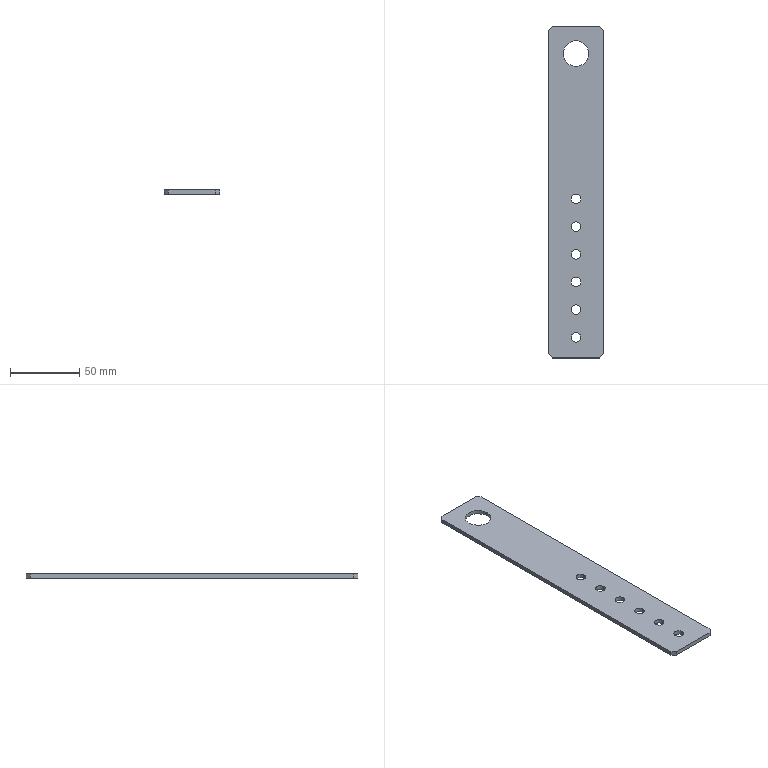Part | SolidWorks | features Extrusion 1 | 1 solid | 24 faces | box 40 x 240 x 3 mm | volume 27247 mm3 | cylinder 14 | plane 10 | commonest cylinder face diameters 7 x12 18.5 x2
STEP:
#1=CARTESIAN_POINT('',(-3.5,-5.,1.5));
#2=VERTEX_POINT('',#1);
#3=CARTESIAN_POINT('',(3.5,-5.,1.5));
#4=VERTEX_POINT('',#3);
#5=CARTESIAN_POINT('',(0.,-5.,1.5));
#6=DIRECTION('',(0.,0.,1.));
#7=DIRECTION('',(1.,0.,0.));
#8=AXIS2_PLACEMENT_3D('',#5,#6,#7);
#9=CIRCLE('',#8,3.5);
#10=EDGE_CURVE('',#2,#4,#9,.T.);
#11=ORIENTED_EDGE('',*,*,#10,.T.);
#12=CARTESIAN_POINT('',(3.5,-5.,-1.5));
#13=VERTEX_POINT('',#12);
#14=CARTESIAN_POINT('',(3.5,-5.,1.5));
#15=DIRECTION('',(0.,0.,-1.));
#16=VECTOR('',#15,1000.);
#17=LINE('',#14,#16);
#18=EDGE_CURVE('',#4,#13,#17,.T.);
#19=ORIENTED_EDGE('',*,*,#18,.T.);
#20=CARTESIAN_POINT('',(-3.5,-5.,-1.5));
#21=VERTEX_POINT('',#20);
#22=CARTESIAN_POINT('',(0.,-5.,-1.5));
#23=DIRECTION('',(0.,0.,1.));
#24=DIRECTION('',(1.,0.,0.));
#25=AXIS2_PLACEMENT_3D('',#22,#23,#24);
#26=CIRCLE('',#25,3.5);
#27=EDGE_CURVE('',#21,#13,#26,.T.);
#28=ORIENTED_EDGE('',*,*,#27,.F.);
#29=CARTESIAN_POINT('',(-3.5,-5.,1.5));
#30=DIRECTION('',(0.,0.,-1.));
#31=VECTOR('',#30,1000.);
#32=LINE('',#29,#31);
#33=EDGE_CURVE('',#2,#21,#32,.T.);
#34=ORIENTED_EDGE('',*,*,#33,.F.);
#35=EDGE_LOOP('',(#11,#19,#28,#34));
#36=FACE_OUTER_BOUND('',#35,.T.);
#37=CARTESIAN_POINT('',(0.,-5.,1.5));
#38=DIRECTION('',(0.,0.,-1.));
#39=DIRECTION('',(-1.,0.,0.));
#40=AXIS2_PLACEMENT_3D('',#37,#38,#39);
#41=CYLINDRICAL_SURFACE('',#40,3.5);
#42=ADVANCED_FACE('',(#36),#41,.F.);
#43=CARTESIAN_POINT('',(-3.5,-25.,1.5));
#44=VERTEX_POINT('',#43);
#45=CARTESIAN_POINT('',(3.5,-25.,1.5));
#46=VERTEX_POINT('',#45);
#47=CARTESIAN_POINT('',(0.,-25.,1.5));
#48=DIRECTION('',(0.,0.,1.));
#49=DIRECTION('',(1.,0.,0.));
#50=AXIS2_PLACEMENT_3D('',#47,#48,#49);
#51=CIRCLE('',#50,3.5);
#52=EDGE_CURVE('',#44,#46,#51,.T.);
#53=ORIENTED_EDGE('',*,*,#52,.T.);
#54=CARTESIAN_POINT('',(3.5,-25.,-1.5));
#55=VERTEX_POINT('',#54);
#56=CARTESIAN_POINT('',(3.5,-25.,1.5));
#57=DIRECTION('',(0.,0.,-1.));
#58=VECTOR('',#57,1000.);
#59=LINE('',#56,#58);
#60=EDGE_CURVE('',#46,#55,#59,.T.);
#61=ORIENTED_EDGE('',*,*,#60,.T.);
#62=CARTESIAN_POINT('',(-3.5,-25.,-1.5));
#63=VERTEX_POINT('',#62);
#64=CARTESIAN_POINT('',(0.,-25.,-1.5));
#65=DIRECTION('',(0.,0.,1.));
#66=DIRECTION('',(1.,0.,0.));
#67=AXIS2_PLACEMENT_3D('',#64,#65,#66);
#68=CIRCLE('',#67,3.5);
#69=EDGE_CURVE('',#63,#55,#68,.T.);
#70=ORIENTED_EDGE('',*,*,#69,.F.);
#71=CARTESIAN_POINT('',(-3.5,-25.,1.5));
#72=DIRECTION('',(0.,0.,-1.));
#73=VECTOR('',#72,1000.);
#74=LINE('',#71,#73);
#75=EDGE_CURVE('',#44,#63,#74,.T.);
#76=ORIENTED_EDGE('',*,*,#75,.F.);
#77=EDGE_LOOP('',(#53,#61,#70,#76));
#78=FACE_OUTER_BOUND('',#77,.T.);
#79=CARTESIAN_POINT('',(0.,-25.,1.5));
#80=DIRECTION('',(0.,0.,-1.));
#81=DIRECTION('',(-1.,0.,0.));
#82=AXIS2_PLACEMENT_3D('',#79,#80,#81);
#83=CYLINDRICAL_SURFACE('',#82,3.5);
#84=ADVANCED_FACE('',(#78),#83,.F.);
#85=CARTESIAN_POINT('',(-3.5,-45.,1.5));
#86=VERTEX_POINT('',#85);
#87=CARTESIAN_POINT('',(3.5,-45.,1.5));
#88=VERTEX_POINT('',#87);
#89=CARTESIAN_POINT('',(0.,-45.,1.5));
#90=DIRECTION('',(0.,0.,1.));
#91=DIRECTION('',(1.,0.,0.));
#92=AXIS2_PLACEMENT_3D('',#89,#90,#91);
#93=CIRCLE('',#92,3.5);
#94=EDGE_CURVE('',#86,#88,#93,.T.);
#95=ORIENTED_EDGE('',*,*,#94,.T.);
#96=CARTESIAN_POINT('',(3.5,-45.,-1.5));
#97=VERTEX_POINT('',#96);
#98=CARTESIAN_POINT('',(3.5,-45.,1.5));
#99=DIRECTION('',(0.,0.,-1.));
#100=VECTOR('',#99,1000.);
#101=LINE('',#98,#100);
#102=EDGE_CURVE('',#88,#97,#101,.T.);
#103=ORIENTED_EDGE('',*,*,#102,.T.);
#104=CARTESIAN_POINT('',(-3.5,-45.,-1.5));
#105=VERTEX_POINT('',#104);
#106=CARTESIAN_POINT('',(0.,-45.,-1.5));
#107=DIRECTION('',(0.,0.,1.));
#108=DIRECTION('',(1.,0.,0.));
#109=AXIS2_PLACEMENT_3D('',#106,#107,#108);
#110=CIRCLE('',#109,3.5);
#111=EDGE_CURVE('',#105,#97,#110,.T.);
#112=ORIENTED_EDGE('',*,*,#111,.F.);
#113=CARTESIAN_POINT('',(-3.5,-45.,1.5));
#114=DIRECTION('',(0.,0.,-1.));
#115=VECTOR('',#114,1000.);
#116=LINE('',#113,#115);
#117=EDGE_CURVE('',#86,#105,#116,.T.);
#118=ORIENTED_EDGE('',*,*,#117,.F.);
#119=EDGE_LOOP('',(#95,#103,#112,#118));
#120=FACE_OUTER_BOUND('',#119,.T.);
#121=CARTESIAN_POINT('',(0.,-45.,1.5));
#122=DIRECTION('',(0.,0.,-1.));
#123=DIRECTION('',(-1.,0.,0.));
#124=AXIS2_PLACEMENT_3D('',#121,#122,#123);
#125=CYLINDRICAL_SURFACE('',#124,3.5);
#126=ADVANCED_FACE('',(#120),#125,.F.);
#127=CARTESIAN_POINT('',(-3.5,-65.,1.5));
#128=VERTEX_POINT('',#127);
#129=CARTESIAN_POINT('',(3.5,-65.,1.5));
#130=VERTEX_POINT('',#129);
#131=CARTESIAN_POINT('',(0.,-65.,1.5));
#132=DIRECTION('',(0.,0.,1.));
#133=DIRECTION('',(1.,0.,0.));
#134=AXIS2_PLACEMENT_3D('',#131,#132,#133);
#135=CIRCLE('',#134,3.5);
#136=EDGE_CURVE('',#128,#130,#135,.T.);
#137=ORIENTED_EDGE('',*,*,#136,.T.);
#138=CARTESIAN_POINT('',(3.5,-65.,-1.5));
#139=VERTEX_POINT('',#138);
#140=CARTESIAN_POINT('',(3.5,-65.,1.5));
#141=DIRECTION('',(0.,0.,-1.));
#142=VECTOR('',#141,1000.);
#143=LINE('',#140,#142);
#144=EDGE_CURVE('',#130,#139,#143,.T.);
#145=ORIENTED_EDGE('',*,*,#144,.T.);
#146=CARTESIAN_POINT('',(-3.5,-65.,-1.5));
#147=VERTEX_POINT('',#146);
#148=CARTESIAN_POINT('',(0.,-65.,-1.5));
#149=DIRECTION('',(0.,0.,1.));
#150=DIRECTION('',(1.,0.,0.));
#151=AXIS2_PLACEMENT_3D('',#148,#149,#150);
#152=CIRCLE('',#151,3.5);
#153=EDGE_CURVE('',#147,#139,#152,.T.);
#154=ORIENTED_EDGE('',*,*,#153,.F.);
#155=CARTESIAN_POINT('',(-3.5,-65.,1.5));
#156=DIRECTION('',(0.,0.,-1.));
#157=VECTOR('',#156,1000.);
#158=LINE('',#155,#157);
#159=EDGE_CURVE('',#128,#147,#158,.T.);
#160=ORIENTED_EDGE('',*,*,#159,.F.);
#161=EDGE_LOOP('',(#137,#145,#154,#160));
#162=FACE_OUTER_BOUND('',#161,.T.);
#163=CARTESIAN_POINT('',(0.,-65.,1.5));
#164=DIRECTION('',(0.,0.,-1.));
#165=DIRECTION('',(-1.,0.,0.));
#166=AXIS2_PLACEMENT_3D('',#163,#164,#165);
#167=CYLINDRICAL_SURFACE('',#166,3.5);
#168=ADVANCED_FACE('',(#162),#167,.F.);
#169=CARTESIAN_POINT('',(-3.5,-85.,1.5));
#170=VERTEX_POINT('',#169);
#171=CARTESIAN_POINT('',(3.5,-85.,1.5));
#172=VERTEX_POINT('',#171);
#173=CARTESIAN_POINT('',(0.,-85.,1.5));
#174=DIRECTION('',(0.,0.,1.));
#175=DIRECTION('',(1.,0.,0.));
#176=AXIS2_PLACEMENT_3D('',#173,#174,#175);
#177=CIRCLE('',#176,3.5);
#178=EDGE_CURVE('',#170,#172,#177,.T.);
#179=ORIENTED_EDGE('',*,*,#178,.T.);
#180=CARTESIAN_POINT('',(3.5,-85.,-1.5));
#181=VERTEX_POINT('',#180);
#182=CARTESIAN_POINT('',(3.5,-85.,1.5));
#183=DIRECTION('',(0.,0.,-1.));
#184=VECTOR('',#183,1000.);
#185=LINE('',#182,#184);
#186=EDGE_CURVE('',#172,#181,#185,.T.);
#187=ORIENTED_EDGE('',*,*,#186,.T.);
#188=CARTESIAN_POINT('',(-3.5,-85.,-1.5));
#189=VERTEX_POINT('',#188);
#190=CARTESIAN_POINT('',(0.,-85.,-1.5));
#191=DIRECTION('',(0.,0.,1.));
#192=DIRECTION('',(1.,0.,0.));
#193=AXIS2_PLACEMENT_3D('',#190,#191,#192);
#194=CIRCLE('',#193,3.5);
#195=EDGE_CURVE('',#189,#181,#194,.T.);
#196=ORIENTED_EDGE('',*,*,#195,.F.);
#197=CARTESIAN_POINT('',(-3.5,-85.,1.5));
#198=DIRECTION('',(0.,0.,-1.));
#199=VECTOR('',#198,1000.);
#200=LINE('',#197,#199);
#201=EDGE_CURVE('',#170,#189,#200,.T.);
#202=ORIENTED_EDGE('',*,*,#201,.F.);
#203=EDGE_LOOP('',(#179,#187,#196,#202));
#204=FACE_OUTER_BOUND('',#203,.T.);
#205=CARTESIAN_POINT('',(0.,-85.,1.5));
#206=DIRECTION('',(0.,0.,-1.));
#207=DIRECTION('',(-1.,0.,0.));
#208=AXIS2_PLACEMENT_3D('',#205,#206,#207);
#209=CYLINDRICAL_SURFACE('',#208,3.5);
#210=ADVANCED_FACE('',(#204),#209,.F.);
#211=CARTESIAN_POINT('',(-3.5,-105.,1.5));
#212=VERTEX_POINT('',#211);
#213=CARTESIAN_POINT('',(3.5,-105.,1.5));
#214=VERTEX_POINT('',#213);
#215=CARTESIAN_POINT('',(0.,-105.,1.5));
#216=DIRECTION('',(0.,0.,1.));
#217=DIRECTION('',(1.,0.,0.));
#218=AXIS2_PLACEMENT_3D('',#215,#216,#217);
#219=CIRCLE('',#218,3.5);
#220=EDGE_CURVE('',#212,#214,#219,.T.);
#221=ORIENTED_EDGE('',*,*,#220,.T.);
#222=CARTESIAN_POINT('',(3.5,-105.,-1.5));
#223=VERTEX_POINT('',#222);
#224=CARTESIAN_POINT('',(3.5,-105.,1.5));
#225=DIRECTION('',(0.,0.,-1.));
#226=VECTOR('',#225,1000.);
#227=LINE('',#224,#226);
#228=EDGE_CURVE('',#214,#223,#227,.T.);
#229=ORIENTED_EDGE('',*,*,#228,.T.);
#230=CARTESIAN_POINT('',(-3.5,-105.,-1.5));
#231=VERTEX_POINT('',#230);
#232=CARTESIAN_POINT('',(0.,-105.,-1.5));
#233=DIRECTION('',(0.,0.,1.));
#234=DIRECTION('',(1.,0.,0.));
#235=AXIS2_PLACEMENT_3D('',#232,#233,#234);
#236=CIRCLE('',#235,3.5);
#237=EDGE_CURVE('',#231,#223,#236,.T.);
#238=ORIENTED_EDGE('',*,*,#237,.F.);
#239=CARTESIAN_POINT('',(-3.5,-105.,1.5));
#240=DIRECTION('',(0.,0.,-1.));
#241=VECTOR('',#240,1000.);
#242=LINE('',#239,#241);
#243=EDGE_CURVE('',#212,#231,#242,.T.);
#244=ORIENTED_EDGE('',*,*,#243,.F.);
#245=EDGE_LOOP('',(#221,#229,#238,#244));
#246=FACE_OUTER_BOUND('',#245,.T.);
#247=CARTESIAN_POINT('',(0.,-105.,1.5));
#248=DIRECTION('',(0.,0.,-1.));
#249=DIRECTION('',(-1.,0.,0.));
#250=AXIS2_PLACEMENT_3D('',#247,#248,#249);
#251=CYLINDRICAL_SURFACE('',#250,3.5);
#252=ADVANCED_FACE('',(#246),#251,.F.);
#253=CARTESIAN_POINT('',(-9.25,100.,1.5));
#254=VERTEX_POINT('',#253);
#255=CARTESIAN_POINT('',(9.25,100.,1.5));
#256=VERTEX_POINT('',#255);
#257=CARTESIAN_POINT('',(0.,100.,1.5));
#258=DIRECTION('',(0.,0.,1.));
#259=DIRECTION('',(1.,0.,0.));
#260=AXIS2_PLACEMENT_3D('',#257,#258,#259);
#261=CIRCLE('',#260,9.25);
#262=EDGE_CURVE('',#254,#256,#261,.T.);
#263=ORIENTED_EDGE('',*,*,#262,.T.);
#264=CARTESIAN_POINT('',(9.25,100.,-1.5));
#265=VERTEX_POINT('',#264);
#266=CARTESIAN_POINT('',(9.25,100.,1.5));
#267=DIRECTION('',(0.,0.,-1.));
#268=VECTOR('',#267,1000.);
#269=LINE('',#266,#268);
#270=EDGE_CURVE('',#256,#265,#269,.T.);
#271=ORIENTED_EDGE('',*,*,#270,.T.);
#272=CARTESIAN_POINT('',(-9.25,100.,-1.5));
#273=VERTEX_POINT('',#272);
#274=CARTESIAN_POINT('',(0.,100.,-1.5));
#275=DIRECTION('',(0.,0.,1.));
#276=DIRECTION('',(1.,0.,0.));
#277=AXIS2_PLACEMENT_3D('',#274,#275,#276);
#278=CIRCLE('',#277,9.25);
#279=EDGE_CURVE('',#273,#265,#278,.T.);
#280=ORIENTED_EDGE('',*,*,#279,.F.);
#281=CARTESIAN_POINT('',(-9.25,100.,1.5));
#282=DIRECTION('',(0.,0.,-1.));
#283=VECTOR('',#282,1000.);
#284=LINE('',#281,#283);
#285=EDGE_CURVE('',#254,#273,#284,.T.);
#286=ORIENTED_EDGE('',*,*,#285,.F.);
#287=EDGE_LOOP('',(#263,#271,#280,#286));
#288=FACE_OUTER_BOUND('',#287,.T.);
#289=CARTESIAN_POINT('',(0.,100.,1.5));
#290=DIRECTION('',(0.,0.,-1.));
#291=DIRECTION('',(-1.,0.,0.));
#292=AXIS2_PLACEMENT_3D('',#289,#290,#291);
#293=CYLINDRICAL_SURFACE('',#292,9.25);
#294=ADVANCED_FACE('',(#288),#293,.F.);
#295=ORIENTED_EDGE('',*,*,#52,.F.);
#296=CARTESIAN_POINT('',(0.,-25.,1.5));
#297=DIRECTION('',(0.,0.,1.));
#298=DIRECTION('',(1.,0.,0.));
#299=AXIS2_PLACEMENT_3D('',#296,#297,#298);
#300=CIRCLE('',#299,3.5);
#301=EDGE_CURVE('',#46,#44,#300,.T.);
#302=ORIENTED_EDGE('',*,*,#301,.F.);
#303=EDGE_LOOP('',(#295,#302));
#304=FACE_BOUND('',#303,.T.);
#305=ORIENTED_EDGE('',*,*,#136,.F.);
#306=CARTESIAN_POINT('',(0.,-65.,1.5));
#307=DIRECTION('',(0.,0.,1.));
#308=DIRECTION('',(1.,0.,0.));
#309=AXIS2_PLACEMENT_3D('',#306,#307,#308);
#310=CIRCLE('',#309,3.5);
#311=EDGE_CURVE('',#130,#128,#310,.T.);
#312=ORIENTED_EDGE('',*,*,#311,.F.);
#313=EDGE_LOOP('',(#305,#312));
#314=FACE_BOUND('',#313,.T.);
#315=ORIENTED_EDGE('',*,*,#220,.F.);
#316=CARTESIAN_POINT('',(0.,-105.,1.5));
#317=DIRECTION('',(0.,0.,1.));
#318=DIRECTION('',(1.,0.,0.));
#319=AXIS2_PLACEMENT_3D('',#316,#317,#318);
#320=CIRCLE('',#319,3.5);
#321=EDGE_CURVE('',#214,#212,#320,.T.);
#322=ORIENTED_EDGE('',*,*,#321,.F.);
#323=EDGE_LOOP('',(#315,#322));
#324=FACE_BOUND('',#323,.T.);
#325=CARTESIAN_POINT('',(-20.,117.,1.5));
#326=VERTEX_POINT('',#325);
#327=CARTESIAN_POINT('',(-20.,-117.,1.5));
#328=VERTEX_POINT('',#327);
#329=CARTESIAN_POINT('',(-20.,-117.,1.5));
#330=DIRECTION('',(0.,-1.,0.));
#331=VECTOR('',#330,1000.);
#332=LINE('',#329,#331);
#333=EDGE_CURVE('',#326,#328,#332,.T.);
#334=ORIENTED_EDGE('',*,*,#333,.T.);
#335=CARTESIAN_POINT('',(-17.,-120.,1.5));
#336=VERTEX_POINT('',#335);
#337=CARTESIAN_POINT('',(-17.,-120.,1.5));
#338=DIRECTION('',(0.7071,-0.7071,0.));
#339=VECTOR('',#338,1000.);
#340=LINE('',#337,#339);
#341=EDGE_CURVE('',#328,#336,#340,.T.);
#342=ORIENTED_EDGE('',*,*,#341,.T.);
#343=CARTESIAN_POINT('',(17.,-120.,1.5));
#344=VERTEX_POINT('',#343);
#345=CARTESIAN_POINT('',(17.,-120.,1.5));
#346=DIRECTION('',(1.,0.,0.));
#347=VECTOR('',#346,1000.);
#348=LINE('',#345,#347);
#349=EDGE_CURVE('',#336,#344,#348,.T.);
#350=ORIENTED_EDGE('',*,*,#349,.T.);
#351=CARTESIAN_POINT('',(20.,-117.,1.5));
#352=VERTEX_POINT('',#351);
#353=CARTESIAN_POINT('',(17.,-120.,1.5));
#354=DIRECTION('',(0.7071,0.7071,0.));
#355=VECTOR('',#354,1000.);
#356=LINE('',#353,#355);
#357=EDGE_CURVE('',#344,#352,#356,.T.);
#358=ORIENTED_EDGE('',*,*,#357,.T.);
#359=CARTESIAN_POINT('',(20.,117.,1.5));
#360=VERTEX_POINT('',#359);
#361=CARTESIAN_POINT('',(20.,-117.,1.5));
#362=DIRECTION('',(0.,1.,0.));
#363=VECTOR('',#362,1000.);
#364=LINE('',#361,#363);
#365=EDGE_CURVE('',#352,#360,#364,.T.);
#366=ORIENTED_EDGE('',*,*,#365,.T.);
#367=CARTESIAN_POINT('',(17.,120.,1.5));
#368=VERTEX_POINT('',#367);
#369=CARTESIAN_POINT('',(20.,117.,1.5));
#370=DIRECTION('',(-0.7071,0.7071,0.));
#371=VECTOR('',#370,1000.);
#372=LINE('',#369,#371);
#373=EDGE_CURVE('',#360,#368,#372,.T.);
#374=ORIENTED_EDGE('',*,*,#373,.T.);
#375=CARTESIAN_POINT('',(-17.,120.,1.5));
#376=VERTEX_POINT('',#375);
#377=CARTESIAN_POINT('',(17.,120.,1.5));
#378=DIRECTION('',(-1.,0.,0.));
#379=VECTOR('',#378,1000.);
#380=LINE('',#377,#379);
#381=EDGE_CURVE('',#368,#376,#380,.T.);
#382=ORIENTED_EDGE('',*,*,#381,.T.);
#383=CARTESIAN_POINT('',(-20.,117.,1.5));
#384=DIRECTION('',(-0.7071,-0.7071,0.));
#385=VECTOR('',#384,1000.);
#386=LINE('',#383,#385);
#387=EDGE_CURVE('',#376,#326,#386,.T.);
#388=ORIENTED_EDGE('',*,*,#387,.T.);
#389=EDGE_LOOP('',(#334,#342,#350,#358,#366,#374,#382,#388));
#390=FACE_OUTER_BOUND('',#389,.T.);
#391=ORIENTED_EDGE('',*,*,#262,.F.);
#392=CARTESIAN_POINT('',(0.,100.,1.5));
#393=DIRECTION('',(0.,0.,1.));
#394=DIRECTION('',(1.,0.,0.));
#395=AXIS2_PLACEMENT_3D('',#392,#393,#394);
#396=CIRCLE('',#395,9.25);
#397=EDGE_CURVE('',#256,#254,#396,.T.);
#398=ORIENTED_EDGE('',*,*,#397,.F.);
#399=EDGE_LOOP('',(#391,#398));
#400=FACE_BOUND('',#399,.T.);
#401=ORIENTED_EDGE('',*,*,#178,.F.);
#402=CARTESIAN_POINT('',(0.,-85.,1.5));
#403=DIRECTION('',(0.,0.,1.));
#404=DIRECTION('',(1.,0.,0.));
#405=AXIS2_PLACEMENT_3D('',#402,#403,#404);
#406=CIRCLE('',#405,3.5);
#407=EDGE_CURVE('',#172,#170,#406,.T.);
#408=ORIENTED_EDGE('',*,*,#407,.F.);
#409=EDGE_LOOP('',(#401,#408));
#410=FACE_BOUND('',#409,.T.);
#411=ORIENTED_EDGE('',*,*,#94,.F.);
#412=CARTESIAN_POINT('',(0.,-45.,1.5));
#413=DIRECTION('',(0.,0.,1.));
#414=DIRECTION('',(1.,0.,0.));
#415=AXIS2_PLACEMENT_3D('',#412,#413,#414);
#416=CIRCLE('',#415,3.5);
#417=EDGE_CURVE('',#88,#86,#416,.T.);
#418=ORIENTED_EDGE('',*,*,#417,.F.);
#419=EDGE_LOOP('',(#411,#418));
#420=FACE_BOUND('',#419,.T.);
#421=ORIENTED_EDGE('',*,*,#10,.F.);
#422=CARTESIAN_POINT('',(0.,-5.,1.5));
#423=DIRECTION('',(0.,0.,1.));
#424=DIRECTION('',(1.,0.,0.));
#425=AXIS2_PLACEMENT_3D('',#422,#423,#424);
#426=CIRCLE('',#425,3.5);
#427=EDGE_CURVE('',#4,#2,#426,.T.);
#428=ORIENTED_EDGE('',*,*,#427,.F.);
#429=EDGE_LOOP('',(#421,#428));
#430=FACE_BOUND('',#429,.T.);
#431=CARTESIAN_POINT('',(0.,0.,1.5));
#432=DIRECTION('',(0.,0.,1.));
#433=DIRECTION('',(1.,0.,0.));
#434=AXIS2_PLACEMENT_3D('',#431,#432,#433);
#435=PLANE('',#434);
#436=ADVANCED_FACE('',(#304,#314,#324,#390,#400,#410,#420,#430),#435,.T.);
#437=CARTESIAN_POINT('',(-20.,117.,-1.5));
#438=VERTEX_POINT('',#437);
#439=CARTESIAN_POINT('',(-20.,-117.,-1.5));
#440=VERTEX_POINT('',#439);
#441=CARTESIAN_POINT('',(-20.,-117.,-1.5));
#442=DIRECTION('',(0.,-1.,0.));
#443=VECTOR('',#442,1000.);
#444=LINE('',#441,#443);
#445=EDGE_CURVE('',#438,#440,#444,.T.);
#446=ORIENTED_EDGE('',*,*,#445,.F.);
#447=CARTESIAN_POINT('',(-17.,120.,-1.5));
#448=VERTEX_POINT('',#447);
#449=CARTESIAN_POINT('',(-20.,117.,-1.5));
#450=DIRECTION('',(-0.7071,-0.7071,0.));
#451=VECTOR('',#450,1000.);
#452=LINE('',#449,#451);
#453=EDGE_CURVE('',#448,#438,#452,.T.);
#454=ORIENTED_EDGE('',*,*,#453,.F.);
#455=CARTESIAN_POINT('',(17.,120.,-1.5));
#456=VERTEX_POINT('',#455);
#457=CARTESIAN_POINT('',(17.,120.,-1.5));
#458=DIRECTION('',(-1.,0.,0.));
#459=VECTOR('',#458,1000.);
#460=LINE('',#457,#459);
#461=EDGE_CURVE('',#456,#448,#460,.T.);
#462=ORIENTED_EDGE('',*,*,#461,.F.);
#463=CARTESIAN_POINT('',(20.,117.,-1.5));
#464=VERTEX_POINT('',#463);
#465=CARTESIAN_POINT('',(20.,117.,-1.5));
#466=DIRECTION('',(-0.7071,0.7071,0.));
#467=VECTOR('',#466,1000.);
#468=LINE('',#465,#467);
#469=EDGE_CURVE('',#464,#456,#468,.T.);
#470=ORIENTED_EDGE('',*,*,#469,.F.);
#471=CARTESIAN_POINT('',(20.,-117.,-1.5));
#472=VERTEX_POINT('',#471);
#473=CARTESIAN_POINT('',(20.,-117.,-1.5));
#474=DIRECTION('',(0.,1.,0.));
#475=VECTOR('',#474,1000.);
#476=LINE('',#473,#475);
#477=EDGE_CURVE('',#472,#464,#476,.T.);
#478=ORIENTED_EDGE('',*,*,#477,.F.);
#479=CARTESIAN_POINT('',(17.,-120.,-1.5));
#480=VERTEX_POINT('',#479);
#481=CARTESIAN_POINT('',(17.,-120.,-1.5));
#482=DIRECTION('',(0.7071,0.7071,0.));
#483=VECTOR('',#482,1000.);
#484=LINE('',#481,#483);
#485=EDGE_CURVE('',#480,#472,#484,.T.);
#486=ORIENTED_EDGE('',*,*,#485,.F.);
#487=CARTESIAN_POINT('',(-17.,-120.,-1.5));
#488=VERTEX_POINT('',#487);
#489=CARTESIAN_POINT('',(17.,-120.,-1.5));
#490=DIRECTION('',(1.,0.,0.));
#491=VECTOR('',#490,1000.);
#492=LINE('',#489,#491);
#493=EDGE_CURVE('',#488,#480,#492,.T.);
#494=ORIENTED_EDGE('',*,*,#493,.F.);
#495=CARTESIAN_POINT('',(-17.,-120.,-1.5));
#496=DIRECTION('',(0.7071,-0.7071,0.));
#497=VECTOR('',#496,1000.);
#498=LINE('',#495,#497);
#499=EDGE_CURVE('',#440,#488,#498,.T.);
#500=ORIENTED_EDGE('',*,*,#499,.F.);
#501=EDGE_LOOP('',(#446,#454,#462,#470,#478,#486,#494,#500));
#502=FACE_OUTER_BOUND('',#501,.T.);
#503=ORIENTED_EDGE('',*,*,#279,.T.);
#504=CARTESIAN_POINT('',(0.,100.,-1.5));
#505=DIRECTION('',(0.,0.,1.));
#506=DIRECTION('',(1.,0.,0.));
#507=AXIS2_PLACEMENT_3D('',#504,#505,#506);
#508=CIRCLE('',#507,9.25);
#509=EDGE_CURVE('',#265,#273,#508,.T.);
#510=ORIENTED_EDGE('',*,*,#509,.T.);
#511=EDGE_LOOP('',(#503,#510));
#512=FACE_BOUND('',#511,.T.);
#513=ORIENTED_EDGE('',*,*,#237,.T.);
#514=CARTESIAN_POINT('',(0.,-105.,-1.5));
#515=DIRECTION('',(0.,0.,1.));
#516=DIRECTION('',(1.,0.,0.));
#517=AXIS2_PLACEMENT_3D('',#514,#515,#516);
#518=CIRCLE('',#517,3.5);
#519=EDGE_CURVE('',#223,#231,#518,.T.);
#520=ORIENTED_EDGE('',*,*,#519,.T.);
#521=EDGE_LOOP('',(#513,#520));
#522=FACE_BOUND('',#521,.T.);
#523=ORIENTED_EDGE('',*,*,#195,.T.);
#524=CARTESIAN_POINT('',(0.,-85.,-1.5));
#525=DIRECTION('',(0.,0.,1.));
#526=DIRECTION('',(1.,0.,0.));
#527=AXIS2_PLACEMENT_3D('',#524,#525,#526);
#528=CIRCLE('',#527,3.5);
#529=EDGE_CURVE('',#181,#189,#528,.T.);
#530=ORIENTED_EDGE('',*,*,#529,.T.);
#531=EDGE_LOOP('',(#523,#530));
#532=FACE_BOUND('',#531,.T.);
#533=ORIENTED_EDGE('',*,*,#153,.T.);
#534=CARTESIAN_POINT('',(0.,-65.,-1.5));
#535=DIRECTION('',(0.,0.,1.));
#536=DIRECTION('',(1.,0.,0.));
#537=AXIS2_PLACEMENT_3D('',#534,#535,#536);
#538=CIRCLE('',#537,3.5);
#539=EDGE_CURVE('',#139,#147,#538,.T.);
#540=ORIENTED_EDGE('',*,*,#539,.T.);
#541=EDGE_LOOP('',(#533,#540));
#542=FACE_BOUND('',#541,.T.);
#543=ORIENTED_EDGE('',*,*,#111,.T.);
#544=CARTESIAN_POINT('',(0.,-45.,-1.5));
#545=DIRECTION('',(0.,0.,1.));
#546=DIRECTION('',(1.,0.,0.));
#547=AXIS2_PLACEMENT_3D('',#544,#545,#546);
#548=CIRCLE('',#547,3.5);
#549=EDGE_CURVE('',#97,#105,#548,.T.);
#550=ORIENTED_EDGE('',*,*,#549,.T.);
#551=EDGE_LOOP('',(#543,#550));
#552=FACE_BOUND('',#551,.T.);
#553=ORIENTED_EDGE('',*,*,#69,.T.);
#554=CARTESIAN_POINT('',(0.,-25.,-1.5));
#555=DIRECTION('',(0.,0.,1.));
#556=DIRECTION('',(1.,0.,0.));
#557=AXIS2_PLACEMENT_3D('',#554,#555,#556);
#558=CIRCLE('',#557,3.5);
#559=EDGE_CURVE('',#55,#63,#558,.T.);
#560=ORIENTED_EDGE('',*,*,#559,.T.);
#561=EDGE_LOOP('',(#553,#560));
#562=FACE_BOUND('',#561,.T.);
#563=ORIENTED_EDGE('',*,*,#27,.T.);
#564=CARTESIAN_POINT('',(0.,-5.,-1.5));
#565=DIRECTION('',(0.,0.,1.));
#566=DIRECTION('',(1.,0.,0.));
#567=AXIS2_PLACEMENT_3D('',#564,#565,#566);
#568=CIRCLE('',#567,3.5);
#569=EDGE_CURVE('',#13,#21,#568,.T.);
#570=ORIENTED_EDGE('',*,*,#569,.T.);
#571=EDGE_LOOP('',(#563,#570));
#572=FACE_BOUND('',#571,.T.);
#573=CARTESIAN_POINT('',(0.,0.,-1.5));
#574=DIRECTION('',(0.,0.,1.));
#575=DIRECTION('',(1.,0.,0.));
#576=AXIS2_PLACEMENT_3D('',#573,#574,#575);
#577=PLANE('',#576);
#578=ADVANCED_FACE('',(#502,#512,#522,#532,#542,#552,#562,#572),#577,.F.);
#579=ORIENTED_EDGE('',*,*,#445,.T.);
#580=CARTESIAN_POINT('',(-20.,-117.,1.5));
#581=DIRECTION('',(0.,0.,-1.));
#582=VECTOR('',#581,1000.);
#583=LINE('',#580,#582);
#584=EDGE_CURVE('',#328,#440,#583,.T.);
#585=ORIENTED_EDGE('',*,*,#584,.F.);
#586=ORIENTED_EDGE('',*,*,#333,.F.);
#587=CARTESIAN_POINT('',(-20.,117.,1.5));
#588=DIRECTION('',(0.,0.,-1.));
#589=VECTOR('',#588,1000.);
#590=LINE('',#587,#589);
#591=EDGE_CURVE('',#326,#438,#590,.T.);
#592=ORIENTED_EDGE('',*,*,#591,.T.);
#593=EDGE_LOOP('',(#579,#585,#586,#592));
#594=FACE_OUTER_BOUND('',#593,.T.);
#595=CARTESIAN_POINT('',(-20.,-117.,1.5));
#596=DIRECTION('',(1.,0.,0.));
#597=DIRECTION('',(0.,0.,-1.));
#598=AXIS2_PLACEMENT_3D('',#595,#596,#597);
#599=PLANE('',#598);
#600=ADVANCED_FACE('',(#594),#599,.F.);
#601=ORIENTED_EDGE('',*,*,#499,.T.);
#602=CARTESIAN_POINT('',(-17.,-120.,1.5));
#603=DIRECTION('',(0.,0.,-1.));
#604=VECTOR('',#603,1000.);
#605=LINE('',#602,#604);
#606=EDGE_CURVE('',#336,#488,#605,.T.);
#607=ORIENTED_EDGE('',*,*,#606,.F.);
#608=ORIENTED_EDGE('',*,*,#341,.F.);
#609=ORIENTED_EDGE('',*,*,#584,.T.);
#610=EDGE_LOOP('',(#601,#607,#608,#609));
#611=FACE_OUTER_BOUND('',#610,.T.);
#612=CARTESIAN_POINT('',(-17.,-120.,1.5));
#613=DIRECTION('',(0.7071,0.7071,0.));
#614=DIRECTION('',(-0.7071,0.7071,0.));
#615=AXIS2_PLACEMENT_3D('',#612,#613,#614);
#616=PLANE('',#615);
#617=ADVANCED_FACE('',(#611),#616,.F.);
#618=ORIENTED_EDGE('',*,*,#493,.T.);
#619=CARTESIAN_POINT('',(17.,-120.,1.5));
#620=DIRECTION('',(0.,0.,-1.));
#621=VECTOR('',#620,1000.);
#622=LINE('',#619,#621);
#623=EDGE_CURVE('',#344,#480,#622,.T.);
#624=ORIENTED_EDGE('',*,*,#623,.F.);
#625=ORIENTED_EDGE('',*,*,#349,.F.);
#626=ORIENTED_EDGE('',*,*,#606,.T.);
#627=EDGE_LOOP('',(#618,#624,#625,#626));
#628=FACE_OUTER_BOUND('',#627,.T.);
#629=CARTESIAN_POINT('',(17.,-120.,1.5));
#630=DIRECTION('',(0.,1.,0.));
#631=DIRECTION('',(0.,0.,1.));
#632=AXIS2_PLACEMENT_3D('',#629,#630,#631);
#633=PLANE('',#632);
#634=ADVANCED_FACE('',(#628),#633,.F.);
#635=ORIENTED_EDGE('',*,*,#485,.T.);
#636=CARTESIAN_POINT('',(20.,-117.,1.5));
#637=DIRECTION('',(0.,0.,-1.));
#638=VECTOR('',#637,1000.);
#639=LINE('',#636,#638);
#640=EDGE_CURVE('',#352,#472,#639,.T.);
#641=ORIENTED_EDGE('',*,*,#640,.F.);
#642=ORIENTED_EDGE('',*,*,#357,.F.);
#643=ORIENTED_EDGE('',*,*,#623,.T.);
#644=EDGE_LOOP('',(#635,#641,#642,#643));
#645=FACE_OUTER_BOUND('',#644,.T.);
#646=CARTESIAN_POINT('',(17.,-120.,1.5));
#647=DIRECTION('',(-0.7071,0.7071,0.));
#648=DIRECTION('',(-0.7071,-0.7071,0.));
#649=AXIS2_PLACEMENT_3D('',#646,#647,#648);
#650=PLANE('',#649);
#651=ADVANCED_FACE('',(#645),#650,.F.);
#652=ORIENTED_EDGE('',*,*,#477,.T.);
#653=CARTESIAN_POINT('',(20.,117.,1.5));
#654=DIRECTION('',(0.,0.,-1.));
#655=VECTOR('',#654,1000.);
#656=LINE('',#653,#655);
#657=EDGE_CURVE('',#360,#464,#656,.T.);
#658=ORIENTED_EDGE('',*,*,#657,.F.);
#659=ORIENTED_EDGE('',*,*,#365,.F.);
#660=ORIENTED_EDGE('',*,*,#640,.T.);
#661=EDGE_LOOP('',(#652,#658,#659,#660));
#662=FACE_OUTER_BOUND('',#661,.T.);
#663=CARTESIAN_POINT('',(20.,-117.,1.5));
#664=DIRECTION('',(-1.,0.,0.));
#665=DIRECTION('',(0.,0.,1.));
#666=AXIS2_PLACEMENT_3D('',#663,#664,#665);
#667=PLANE('',#666);
#668=ADVANCED_FACE('',(#662),#667,.F.);
#669=ORIENTED_EDGE('',*,*,#469,.T.);
#670=CARTESIAN_POINT('',(17.,120.,1.5));
#671=DIRECTION('',(0.,0.,-1.));
#672=VECTOR('',#671,1000.);
#673=LINE('',#670,#672);
#674=EDGE_CURVE('',#368,#456,#673,.T.);
#675=ORIENTED_EDGE('',*,*,#674,.F.);
#676=ORIENTED_EDGE('',*,*,#373,.F.);
#677=ORIENTED_EDGE('',*,*,#657,.T.);
#678=EDGE_LOOP('',(#669,#675,#676,#677));
#679=FACE_OUTER_BOUND('',#678,.T.);
#680=CARTESIAN_POINT('',(20.,117.,1.5));
#681=DIRECTION('',(-0.7071,-0.7071,0.));
#682=DIRECTION('',(0.7071,-0.7071,0.));
#683=AXIS2_PLACEMENT_3D('',#680,#681,#682);
#684=PLANE('',#683);
#685=ADVANCED_FACE('',(#679),#684,.F.);
#686=ORIENTED_EDGE('',*,*,#461,.T.);
#687=CARTESIAN_POINT('',(-17.,120.,1.5));
#688=DIRECTION('',(0.,0.,-1.));
#689=VECTOR('',#688,1000.);
#690=LINE('',#687,#689);
#691=EDGE_CURVE('',#376,#448,#690,.T.);
#692=ORIENTED_EDGE('',*,*,#691,.F.);
#693=ORIENTED_EDGE('',*,*,#381,.F.);
#694=ORIENTED_EDGE('',*,*,#674,.T.);
#695=EDGE_LOOP('',(#686,#692,#693,#694));
#696=FACE_OUTER_BOUND('',#695,.T.);
#697=CARTESIAN_POINT('',(17.,120.,1.5));
#698=DIRECTION('',(0.,-1.,0.));
#699=DIRECTION('',(1.,0.,0.));
#700=AXIS2_PLACEMENT_3D('',#697,#698,#699);
#701=PLANE('',#700);
#702=ADVANCED_FACE('',(#696),#701,.F.);
#703=ORIENTED_EDGE('',*,*,#453,.T.);
#704=ORIENTED_EDGE('',*,*,#591,.F.);
#705=ORIENTED_EDGE('',*,*,#387,.F.);
#706=ORIENTED_EDGE('',*,*,#691,.T.);
#707=EDGE_LOOP('',(#703,#704,#705,#706));
#708=FACE_OUTER_BOUND('',#707,.T.);
#709=CARTESIAN_POINT('',(-20.,117.,1.5));
#710=DIRECTION('',(0.7071,-0.7071,0.));
#711=DIRECTION('',(0.7071,0.7071,0.));
#712=AXIS2_PLACEMENT_3D('',#709,#710,#711);
#713=PLANE('',#712);
#714=ADVANCED_FACE('',(#708),#713,.F.);
#715=ORIENTED_EDGE('',*,*,#270,.F.);
#716=ORIENTED_EDGE('',*,*,#397,.T.);
#717=ORIENTED_EDGE('',*,*,#285,.T.);
#718=ORIENTED_EDGE('',*,*,#509,.F.);
#719=EDGE_LOOP('',(#715,#716,#717,#718));
#720=FACE_OUTER_BOUND('',#719,.T.);
#721=CARTESIAN_POINT('',(0.,100.,1.5));
#722=DIRECTION('',(0.,0.,-1.));
#723=DIRECTION('',(-1.,0.,0.));
#724=AXIS2_PLACEMENT_3D('',#721,#722,#723);
#725=CYLINDRICAL_SURFACE('',#724,9.25);
#726=ADVANCED_FACE('',(#720),#725,.F.);
#727=ORIENTED_EDGE('',*,*,#228,.F.);
#728=ORIENTED_EDGE('',*,*,#321,.T.);
#729=ORIENTED_EDGE('',*,*,#243,.T.);
#730=ORIENTED_EDGE('',*,*,#519,.F.);
#731=EDGE_LOOP('',(#727,#728,#729,#730));
#732=FACE_OUTER_BOUND('',#731,.T.);
#733=CARTESIAN_POINT('',(0.,-105.,1.5));
#734=DIRECTION('',(0.,0.,-1.));
#735=DIRECTION('',(-1.,0.,0.));
#736=AXIS2_PLACEMENT_3D('',#733,#734,#735);
#737=CYLINDRICAL_SURFACE('',#736,3.5);
#738=ADVANCED_FACE('',(#732),#737,.F.);
#739=ORIENTED_EDGE('',*,*,#186,.F.);
#740=ORIENTED_EDGE('',*,*,#407,.T.);
#741=ORIENTED_EDGE('',*,*,#201,.T.);
#742=ORIENTED_EDGE('',*,*,#529,.F.);
#743=EDGE_LOOP('',(#739,#740,#741,#742));
#744=FACE_OUTER_BOUND('',#743,.T.);
#745=CARTESIAN_POINT('',(0.,-85.,1.5));
#746=DIRECTION('',(0.,0.,-1.));
#747=DIRECTION('',(-1.,0.,0.));
#748=AXIS2_PLACEMENT_3D('',#745,#746,#747);
#749=CYLINDRICAL_SURFACE('',#748,3.5);
#750=ADVANCED_FACE('',(#744),#749,.F.);
#751=ORIENTED_EDGE('',*,*,#144,.F.);
#752=ORIENTED_EDGE('',*,*,#311,.T.);
#753=ORIENTED_EDGE('',*,*,#159,.T.);
#754=ORIENTED_EDGE('',*,*,#539,.F.);
#755=EDGE_LOOP('',(#751,#752,#753,#754));
#756=FACE_OUTER_BOUND('',#755,.T.);
#757=CARTESIAN_POINT('',(0.,-65.,1.5));
#758=DIRECTION('',(0.,0.,-1.));
#759=DIRECTION('',(-1.,0.,0.));
#760=AXIS2_PLACEMENT_3D('',#757,#758,#759);
#761=CYLINDRICAL_SURFACE('',#760,3.5);
#762=ADVANCED_FACE('',(#756),#761,.F.);
#763=ORIENTED_EDGE('',*,*,#102,.F.);
#764=ORIENTED_EDGE('',*,*,#417,.T.);
#765=ORIENTED_EDGE('',*,*,#117,.T.);
#766=ORIENTED_EDGE('',*,*,#549,.F.);
#767=EDGE_LOOP('',(#763,#764,#765,#766));
#768=FACE_OUTER_BOUND('',#767,.T.);
#769=CARTESIAN_POINT('',(0.,-45.,1.5));
#770=DIRECTION('',(0.,0.,-1.));
#771=DIRECTION('',(-1.,0.,0.));
#772=AXIS2_PLACEMENT_3D('',#769,#770,#771);
#773=CYLINDRICAL_SURFACE('',#772,3.5);
#774=ADVANCED_FACE('',(#768),#773,.F.);
#775=ORIENTED_EDGE('',*,*,#60,.F.);
#776=ORIENTED_EDGE('',*,*,#301,.T.);
#777=ORIENTED_EDGE('',*,*,#75,.T.);
#778=ORIENTED_EDGE('',*,*,#559,.F.);
#779=EDGE_LOOP('',(#775,#776,#777,#778));
#780=FACE_OUTER_BOUND('',#779,.T.);
#781=CARTESIAN_POINT('',(0.,-25.,1.5));
#782=DIRECTION('',(0.,0.,-1.));
#783=DIRECTION('',(-1.,0.,0.));
#784=AXIS2_PLACEMENT_3D('',#781,#782,#783);
#785=CYLINDRICAL_SURFACE('',#784,3.5);
#786=ADVANCED_FACE('',(#780),#785,.F.);
#787=ORIENTED_EDGE('',*,*,#18,.F.);
#788=ORIENTED_EDGE('',*,*,#427,.T.);
#789=ORIENTED_EDGE('',*,*,#33,.T.);
#790=ORIENTED_EDGE('',*,*,#569,.F.);
#791=EDGE_LOOP('',(#787,#788,#789,#790));
#792=FACE_OUTER_BOUND('',#791,.T.);
#793=CARTESIAN_POINT('',(0.,-5.,1.5));
#794=DIRECTION('',(0.,0.,-1.));
#795=DIRECTION('',(-1.,0.,0.));
#796=AXIS2_PLACEMENT_3D('',#793,#794,#795);
#797=CYLINDRICAL_SURFACE('',#796,3.5);
#798=ADVANCED_FACE('',(#792),#797,.F.);
#799=CLOSED_SHELL('',(#42,#84,#126,#168,#210,#252,#294,#436,#578,#600,#617,#634,#651,#668,#685,#702,#714,#726,#738,#750,#762,#774,#786,#798));
#800=MANIFOLD_SOLID_BREP('',#799);
#801=CARTESIAN_POINT('',(0.,0.,0.));
#802=DIRECTION('',(0.,0.,1.));
#803=DIRECTION('',(1.,0.,0.));
#804=AXIS2_PLACEMENT_3D('',#801,#802,#803);
#805=(LENGTH_UNIT()NAMED_UNIT(*)SI_UNIT(.MILLI.,.METRE.));
#806=UNCERTAINTY_MEASURE_WITH_UNIT(LENGTH_MEASURE(0.00001),#805,'','');
#807=(NAMED_UNIT(*)PLANE_ANGLE_UNIT()SI_UNIT($,.RADIAN.));
#808=(NAMED_UNIT(*)SI_UNIT($,.STERADIAN.)SOLID_ANGLE_UNIT());
#809=(GEOMETRIC_REPRESENTATION_CONTEXT(3)GLOBAL_UNCERTAINTY_ASSIGNED_CONTEXT((#806))GLOBAL_UNIT_ASSIGNED_CONTEXT((#805,#807,#808))REPRESENTATION_CONTEXT('',''));
#810=ADVANCED_BREP_SHAPE_REPRESENTATION('',(#800,#804),#809);